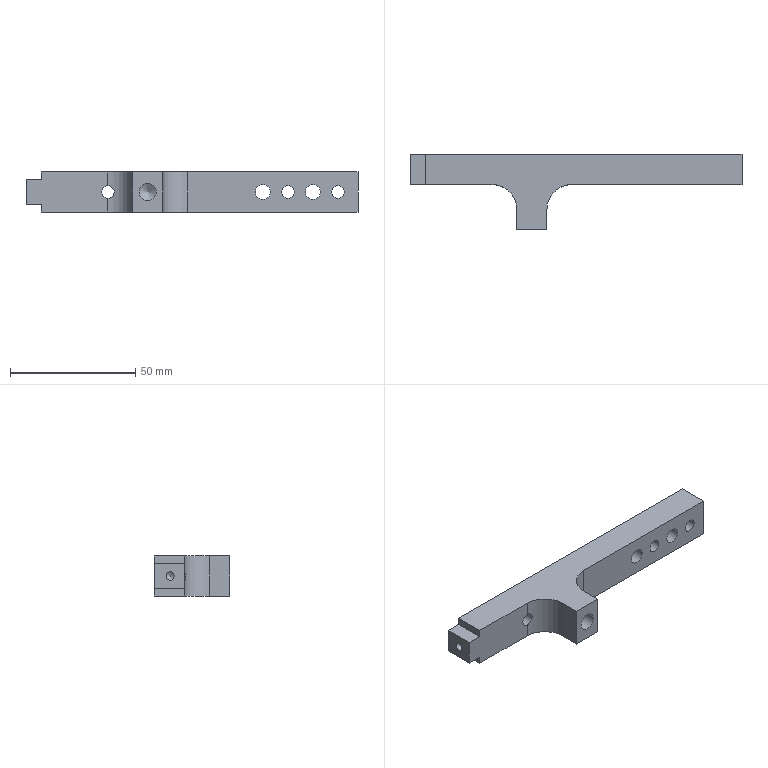Part | NX | features BREP 1 | 1 solid | 25 faces | box 132.75 x 30 x 16 mm | volume 26981 mm3 | plane 14 | cylinder 9 | cone 2 | commonest cylinder face diameters 5 x3 6 x2 20 x2 3.3 x1 6.8 x1
STEP:
#1=CARTESIAN_POINT('',(-36.75,30.,3.));
#2=VERTEX_POINT('',#1);
#3=CARTESIAN_POINT('',(-36.75,30.,0.));
#4=VERTEX_POINT('',#3);
#5=CARTESIAN_POINT('',(-36.75,30.,16.));
#6=DIRECTION('',(0.,0.,-1.));
#7=VECTOR('',#6,1000.);
#8=LINE('',#5,#7);
#9=EDGE_CURVE('',#2,#4,#8,.T.);
#10=ORIENTED_EDGE('',*,*,#9,.F.);
#11=CARTESIAN_POINT('',(-42.75,30.,3.));
#12=VERTEX_POINT('',#11);
#13=CARTESIAN_POINT('',(0.,30.,3.));
#14=DIRECTION('',(1.,0.,0.));
#15=VECTOR('',#14,1000.);
#16=LINE('',#13,#15);
#17=EDGE_CURVE('',#12,#2,#16,.T.);
#18=ORIENTED_EDGE('',*,*,#17,.F.);
#19=CARTESIAN_POINT('',(-42.75,30.,13.));
#20=VERTEX_POINT('',#19);
#21=CARTESIAN_POINT('',(-42.75,30.,16.));
#22=DIRECTION('',(0.,0.,-1.));
#23=VECTOR('',#22,1000.);
#24=LINE('',#21,#23);
#25=EDGE_CURVE('',#20,#12,#24,.T.);
#26=ORIENTED_EDGE('',*,*,#25,.F.);
#27=CARTESIAN_POINT('',(-36.75,30.,13.));
#28=VERTEX_POINT('',#27);
#29=CARTESIAN_POINT('',(0.,30.,13.));
#30=DIRECTION('',(-1.,0.,0.));
#31=VECTOR('',#30,1000.);
#32=LINE('',#29,#31);
#33=EDGE_CURVE('',#28,#20,#32,.T.);
#34=ORIENTED_EDGE('',*,*,#33,.F.);
#35=CARTESIAN_POINT('',(-36.75,30.,16.));
#36=VERTEX_POINT('',#35);
#37=CARTESIAN_POINT('',(-36.75,30.,16.));
#38=DIRECTION('',(0.,0.,-1.));
#39=VECTOR('',#38,1000.);
#40=LINE('',#37,#39);
#41=EDGE_CURVE('',#36,#28,#40,.T.);
#42=ORIENTED_EDGE('',*,*,#41,.F.);
#43=CARTESIAN_POINT('',(90.,30.,16.));
#44=VERTEX_POINT('',#43);
#45=CARTESIAN_POINT('',(0.,30.,16.));
#46=DIRECTION('',(-1.,0.,0.));
#47=VECTOR('',#46,1000.);
#48=LINE('',#45,#47);
#49=EDGE_CURVE('',#44,#36,#48,.T.);
#50=ORIENTED_EDGE('',*,*,#49,.F.);
#51=CARTESIAN_POINT('',(90.,30.,0.));
#52=VERTEX_POINT('',#51);
#53=CARTESIAN_POINT('',(90.,30.,16.));
#54=DIRECTION('',(0.,0.,1.));
#55=VECTOR('',#54,1000.);
#56=LINE('',#53,#55);
#57=EDGE_CURVE('',#52,#44,#56,.T.);
#58=ORIENTED_EDGE('',*,*,#57,.F.);
#59=CARTESIAN_POINT('',(0.,30.,0.));
#60=DIRECTION('',(1.,0.,0.));
#61=VECTOR('',#60,1000.);
#62=LINE('',#59,#61);
#63=EDGE_CURVE('',#4,#52,#62,.T.);
#64=ORIENTED_EDGE('',*,*,#63,.F.);
#65=EDGE_LOOP('',(#10,#18,#26,#34,#42,#50,#58,#64));
#66=FACE_BOUND('',#65,.T.);
#67=CARTESIAN_POINT('',(72.,30.,11.));
#68=VERTEX_POINT('',#67);
#69=CARTESIAN_POINT('',(72.,30.,8.));
#70=DIRECTION('',(0.,1.,0.));
#71=DIRECTION('',(0.,0.,1.));
#72=AXIS2_PLACEMENT_3D('',#69,#70,#71);
#73=CIRCLE('',#72,3.);
#74=EDGE_CURVE('',#68,#68,#73,.T.);
#75=ORIENTED_EDGE('',*,*,#74,.F.);
#76=EDGE_LOOP('',(#75));
#77=FACE_BOUND('',#76,.T.);
#78=CARTESIAN_POINT('',(52.,30.,11.));
#79=VERTEX_POINT('',#78);
#80=CARTESIAN_POINT('',(52.,30.,8.));
#81=DIRECTION('',(0.,1.,0.));
#82=DIRECTION('',(0.,0.,1.));
#83=AXIS2_PLACEMENT_3D('',#80,#81,#82);
#84=CIRCLE('',#83,3.);
#85=EDGE_CURVE('',#79,#79,#84,.T.);
#86=ORIENTED_EDGE('',*,*,#85,.F.);
#87=EDGE_LOOP('',(#86));
#88=FACE_BOUND('',#87,.T.);
#89=CARTESIAN_POINT('',(62.,30.,10.5));
#90=VERTEX_POINT('',#89);
#91=CARTESIAN_POINT('',(62.,30.,8.));
#92=DIRECTION('',(0.,1.,0.));
#93=DIRECTION('',(0.,0.,1.));
#94=AXIS2_PLACEMENT_3D('',#91,#92,#93);
#95=CIRCLE('',#94,2.5);
#96=EDGE_CURVE('',#90,#90,#95,.T.);
#97=ORIENTED_EDGE('',*,*,#96,.F.);
#98=EDGE_LOOP('',(#97));
#99=FACE_BOUND('',#98,.T.);
#100=CARTESIAN_POINT('',(82.,30.,10.5));
#101=VERTEX_POINT('',#100);
#102=CARTESIAN_POINT('',(82.,30.,8.));
#103=DIRECTION('',(0.,1.,0.));
#104=DIRECTION('',(0.,0.,1.));
#105=AXIS2_PLACEMENT_3D('',#102,#103,#104);
#106=CIRCLE('',#105,2.5);
#107=EDGE_CURVE('',#101,#101,#106,.T.);
#108=ORIENTED_EDGE('',*,*,#107,.F.);
#109=EDGE_LOOP('',(#108));
#110=FACE_BOUND('',#109,.T.);
#111=CARTESIAN_POINT('',(-10.,30.,10.5));
#112=VERTEX_POINT('',#111);
#113=CARTESIAN_POINT('',(-10.,30.,8.));
#114=DIRECTION('',(0.,1.,0.));
#115=DIRECTION('',(0.,0.,1.));
#116=AXIS2_PLACEMENT_3D('',#113,#114,#115);
#117=CIRCLE('',#116,2.5);
#118=EDGE_CURVE('',#112,#112,#117,.T.);
#119=ORIENTED_EDGE('',*,*,#118,.F.);
#120=EDGE_LOOP('',(#119));
#121=FACE_BOUND('',#120,.T.);
#122=CARTESIAN_POINT('',(0.,30.,16.));
#123=DIRECTION('',(0.,-1.,0.));
#124=DIRECTION('',(0.,0.,1.));
#125=AXIS2_PLACEMENT_3D('',#122,#123,#124);
#126=PLANE('',#125);
#127=ADVANCED_FACE('',(#66,#77,#88,#99,#110,#121),#126,.F.);
#128=CARTESIAN_POINT('',(0.,8.,0.));
#129=VERTEX_POINT('',#128);
#130=CARTESIAN_POINT('',(-10.,18.,0.));
#131=VERTEX_POINT('',#130);
#132=CARTESIAN_POINT('',(-10.,8.,0.));
#133=DIRECTION('',(0.,0.,1.));
#134=DIRECTION('',(-1.,0.,0.));
#135=AXIS2_PLACEMENT_3D('',#132,#133,#134);
#136=CIRCLE('',#135,10.);
#137=EDGE_CURVE('',#129,#131,#136,.T.);
#138=ORIENTED_EDGE('',*,*,#137,.T.);
#139=CARTESIAN_POINT('',(-36.75,18.,0.));
#140=VERTEX_POINT('',#139);
#141=CARTESIAN_POINT('',(0.,18.,0.));
#142=DIRECTION('',(-1.,0.,0.));
#143=VECTOR('',#142,1000.);
#144=LINE('',#141,#143);
#145=EDGE_CURVE('',#131,#140,#144,.T.);
#146=ORIENTED_EDGE('',*,*,#145,.T.);
#147=CARTESIAN_POINT('',(-36.75,0.,0.));
#148=DIRECTION('',(0.,1.,0.));
#149=VECTOR('',#148,1000.);
#150=LINE('',#147,#149);
#151=EDGE_CURVE('',#140,#4,#150,.T.);
#152=ORIENTED_EDGE('',*,*,#151,.T.);
#153=ORIENTED_EDGE('',*,*,#63,.T.);
#154=CARTESIAN_POINT('',(90.,18.,0.));
#155=VERTEX_POINT('',#154);
#156=CARTESIAN_POINT('',(90.,0.,0.));
#157=DIRECTION('',(0.,-1.,0.));
#158=VECTOR('',#157,1000.);
#159=LINE('',#156,#158);
#160=EDGE_CURVE('',#52,#155,#159,.T.);
#161=ORIENTED_EDGE('',*,*,#160,.T.);
#162=CARTESIAN_POINT('',(22.,18.,0.));
#163=VERTEX_POINT('',#162);
#164=CARTESIAN_POINT('',(0.,18.,0.));
#165=DIRECTION('',(-1.,0.,0.));
#166=VECTOR('',#165,1000.);
#167=LINE('',#164,#166);
#168=EDGE_CURVE('',#155,#163,#167,.T.);
#169=ORIENTED_EDGE('',*,*,#168,.T.);
#170=CARTESIAN_POINT('',(12.,8.,0.));
#171=VERTEX_POINT('',#170);
#172=CARTESIAN_POINT('',(22.,8.,0.));
#173=DIRECTION('',(0.,0.,1.));
#174=DIRECTION('',(1.,0.,0.));
#175=AXIS2_PLACEMENT_3D('',#172,#173,#174);
#176=CIRCLE('',#175,10.);
#177=EDGE_CURVE('',#163,#171,#176,.T.);
#178=ORIENTED_EDGE('',*,*,#177,.T.);
#179=CARTESIAN_POINT('',(12.,0.,0.));
#180=VERTEX_POINT('',#179);
#181=CARTESIAN_POINT('',(12.,0.,0.));
#182=DIRECTION('',(0.,-1.,0.));
#183=VECTOR('',#182,1000.);
#184=LINE('',#181,#183);
#185=EDGE_CURVE('',#171,#180,#184,.T.);
#186=ORIENTED_EDGE('',*,*,#185,.T.);
#187=CARTESIAN_POINT('',(0.,0.,0.));
#188=VERTEX_POINT('',#187);
#189=CARTESIAN_POINT('',(0.,0.,0.));
#190=DIRECTION('',(-1.,0.,0.));
#191=VECTOR('',#190,1000.);
#192=LINE('',#189,#191);
#193=EDGE_CURVE('',#180,#188,#192,.T.);
#194=ORIENTED_EDGE('',*,*,#193,.T.);
#195=CARTESIAN_POINT('',(0.,0.,0.));
#196=DIRECTION('',(0.,1.,0.));
#197=VECTOR('',#196,1000.);
#198=LINE('',#195,#197);
#199=EDGE_CURVE('',#188,#129,#198,.T.);
#200=ORIENTED_EDGE('',*,*,#199,.T.);
#201=EDGE_LOOP('',(#138,#146,#152,#153,#161,#169,#178,#186,#194,#200));
#202=FACE_BOUND('',#201,.T.);
#203=CARTESIAN_POINT('',(0.,0.,0.));
#204=DIRECTION('',(0.,0.,-1.));
#205=DIRECTION('',(1.,0.,0.));
#206=AXIS2_PLACEMENT_3D('',#203,#204,#205);
#207=PLANE('',#206);
#208=ADVANCED_FACE('',(#202),#207,.T.);
#209=CARTESIAN_POINT('',(-36.75,18.,3.));
#210=VERTEX_POINT('',#209);
#211=CARTESIAN_POINT('',(-36.75,0.,3.));
#212=DIRECTION('',(0.,-1.,0.));
#213=VECTOR('',#212,1000.);
#214=LINE('',#211,#213);
#215=EDGE_CURVE('',#2,#210,#214,.T.);
#216=ORIENTED_EDGE('',*,*,#215,.F.);
#217=ORIENTED_EDGE('',*,*,#9,.T.);
#218=ORIENTED_EDGE('',*,*,#151,.F.);
#219=CARTESIAN_POINT('',(-36.75,18.,0.));
#220=DIRECTION('',(0.,0.,-1.));
#221=VECTOR('',#220,1000.);
#222=LINE('',#219,#221);
#223=EDGE_CURVE('',#210,#140,#222,.T.);
#224=ORIENTED_EDGE('',*,*,#223,.F.);
#225=EDGE_LOOP('',(#216,#217,#218,#224));
#226=FACE_BOUND('',#225,.T.);
#227=CARTESIAN_POINT('',(-36.75,0.,0.));
#228=DIRECTION('',(1.,0.,0.));
#229=DIRECTION('',(0.,0.,1.));
#230=AXIS2_PLACEMENT_3D('',#227,#228,#229);
#231=PLANE('',#230);
#232=ADVANCED_FACE('',(#226),#231,.F.);
#233=CARTESIAN_POINT('',(-42.75,18.,3.));
#234=VERTEX_POINT('',#233);
#235=CARTESIAN_POINT('',(-42.75,0.,3.));
#236=DIRECTION('',(0.,-1.,0.));
#237=VECTOR('',#236,1000.);
#238=LINE('',#235,#237);
#239=EDGE_CURVE('',#12,#234,#238,.T.);
#240=ORIENTED_EDGE('',*,*,#239,.F.);
#241=ORIENTED_EDGE('',*,*,#17,.T.);
#242=ORIENTED_EDGE('',*,*,#215,.T.);
#243=CARTESIAN_POINT('',(-36.75,18.,3.));
#244=DIRECTION('',(1.,0.,0.));
#245=VECTOR('',#244,1000.);
#246=LINE('',#243,#245);
#247=EDGE_CURVE('',#234,#210,#246,.T.);
#248=ORIENTED_EDGE('',*,*,#247,.F.);
#249=EDGE_LOOP('',(#240,#241,#242,#248));
#250=FACE_BOUND('',#249,.T.);
#251=CARTESIAN_POINT('',(-36.75,0.,3.));
#252=DIRECTION('',(0.,0.,1.));
#253=DIRECTION('',(-1.,0.,0.));
#254=AXIS2_PLACEMENT_3D('',#251,#252,#253);
#255=PLANE('',#254);
#256=ADVANCED_FACE('',(#250),#255,.F.);
#257=CARTESIAN_POINT('',(-42.75,18.,13.));
#258=VERTEX_POINT('',#257);
#259=CARTESIAN_POINT('',(-42.75,30.,13.));
#260=DIRECTION('',(0.,1.,0.));
#261=VECTOR('',#260,1000.);
#262=LINE('',#259,#261);
#263=EDGE_CURVE('',#258,#20,#262,.T.);
#264=ORIENTED_EDGE('',*,*,#263,.T.);
#265=ORIENTED_EDGE('',*,*,#25,.T.);
#266=ORIENTED_EDGE('',*,*,#239,.T.);
#267=CARTESIAN_POINT('',(-42.75,18.,16.));
#268=DIRECTION('',(0.,0.,1.));
#269=VECTOR('',#268,1000.);
#270=LINE('',#267,#269);
#271=EDGE_CURVE('',#234,#258,#270,.T.);
#272=ORIENTED_EDGE('',*,*,#271,.T.);
#273=EDGE_LOOP('',(#264,#265,#266,#272));
#274=FACE_BOUND('',#273,.T.);
#275=CARTESIAN_POINT('',(-42.75,23.75,9.65));
#276=VERTEX_POINT('',#275);
#277=CARTESIAN_POINT('',(-42.75,23.75,8.));
#278=DIRECTION('',(1.,0.,0.));
#279=DIRECTION('',(0.,0.,1.));
#280=AXIS2_PLACEMENT_3D('',#277,#278,#279);
#281=CIRCLE('',#280,1.65);
#282=EDGE_CURVE('',#276,#276,#281,.T.);
#283=ORIENTED_EDGE('',*,*,#282,.T.);
#284=EDGE_LOOP('',(#283));
#285=FACE_BOUND('',#284,.T.);
#286=CARTESIAN_POINT('',(-42.75,30.,16.));
#287=DIRECTION('',(-1.,0.,0.));
#288=DIRECTION('',(0.,1.,0.));
#289=AXIS2_PLACEMENT_3D('',#286,#287,#288);
#290=PLANE('',#289);
#291=ADVANCED_FACE('',(#274,#285),#290,.T.);
#292=CARTESIAN_POINT('',(-36.75,18.,13.));
#293=VERTEX_POINT('',#292);
#294=CARTESIAN_POINT('',(-36.75,0.,13.));
#295=DIRECTION('',(0.,-1.,0.));
#296=VECTOR('',#295,1000.);
#297=LINE('',#294,#296);
#298=EDGE_CURVE('',#28,#293,#297,.T.);
#299=ORIENTED_EDGE('',*,*,#298,.F.);
#300=ORIENTED_EDGE('',*,*,#33,.T.);
#301=ORIENTED_EDGE('',*,*,#263,.F.);
#302=CARTESIAN_POINT('',(-36.75,18.,13.));
#303=DIRECTION('',(-1.,0.,0.));
#304=VECTOR('',#303,1000.);
#305=LINE('',#302,#304);
#306=EDGE_CURVE('',#293,#258,#305,.T.);
#307=ORIENTED_EDGE('',*,*,#306,.F.);
#308=EDGE_LOOP('',(#299,#300,#301,#307));
#309=FACE_BOUND('',#308,.T.);
#310=CARTESIAN_POINT('',(-36.75,0.,13.));
#311=DIRECTION('',(0.,0.,-1.));
#312=DIRECTION('',(1.,0.,0.));
#313=AXIS2_PLACEMENT_3D('',#310,#311,#312);
#314=PLANE('',#313);
#315=ADVANCED_FACE('',(#309),#314,.F.);
#316=CARTESIAN_POINT('',(-36.75,18.,16.));
#317=VERTEX_POINT('',#316);
#318=CARTESIAN_POINT('',(-36.75,0.,16.));
#319=DIRECTION('',(0.,-1.,0.));
#320=VECTOR('',#319,1000.);
#321=LINE('',#318,#320);
#322=EDGE_CURVE('',#36,#317,#321,.T.);
#323=ORIENTED_EDGE('',*,*,#322,.F.);
#324=ORIENTED_EDGE('',*,*,#41,.T.);
#325=ORIENTED_EDGE('',*,*,#298,.T.);
#326=CARTESIAN_POINT('',(-36.75,18.,16.));
#327=DIRECTION('',(0.,0.,-1.));
#328=VECTOR('',#327,1000.);
#329=LINE('',#326,#328);
#330=EDGE_CURVE('',#317,#293,#329,.T.);
#331=ORIENTED_EDGE('',*,*,#330,.F.);
#332=EDGE_LOOP('',(#323,#324,#325,#331));
#333=FACE_BOUND('',#332,.T.);
#334=CARTESIAN_POINT('',(-36.75,0.,16.));
#335=DIRECTION('',(1.,0.,0.));
#336=DIRECTION('',(0.,0.,1.));
#337=AXIS2_PLACEMENT_3D('',#334,#335,#336);
#338=PLANE('',#337);
#339=ADVANCED_FACE('',(#333),#338,.F.);
#340=ORIENTED_EDGE('',*,*,#322,.T.);
#341=CARTESIAN_POINT('',(-10.,18.,16.));
#342=VERTEX_POINT('',#341);
#343=CARTESIAN_POINT('',(0.,18.,16.));
#344=DIRECTION('',(-1.,0.,0.));
#345=VECTOR('',#344,1000.);
#346=LINE('',#343,#345);
#347=EDGE_CURVE('',#342,#317,#346,.T.);
#348=ORIENTED_EDGE('',*,*,#347,.F.);
#349=CARTESIAN_POINT('',(0.,8.,16.));
#350=VERTEX_POINT('',#349);
#351=CARTESIAN_POINT('',(-10.,8.,16.));
#352=DIRECTION('',(0.,0.,1.));
#353=DIRECTION('',(-1.,0.,0.));
#354=AXIS2_PLACEMENT_3D('',#351,#352,#353);
#355=CIRCLE('',#354,10.);
#356=EDGE_CURVE('',#350,#342,#355,.T.);
#357=ORIENTED_EDGE('',*,*,#356,.F.);
#358=CARTESIAN_POINT('',(0.,0.,16.));
#359=VERTEX_POINT('',#358);
#360=CARTESIAN_POINT('',(0.,0.,16.));
#361=DIRECTION('',(0.,1.,0.));
#362=VECTOR('',#361,1000.);
#363=LINE('',#360,#362);
#364=EDGE_CURVE('',#359,#350,#363,.T.);
#365=ORIENTED_EDGE('',*,*,#364,.F.);
#366=CARTESIAN_POINT('',(12.,0.,16.));
#367=VERTEX_POINT('',#366);
#368=CARTESIAN_POINT('',(0.,0.,16.));
#369=DIRECTION('',(-1.,0.,0.));
#370=VECTOR('',#369,1000.);
#371=LINE('',#368,#370);
#372=EDGE_CURVE('',#367,#359,#371,.T.);
#373=ORIENTED_EDGE('',*,*,#372,.F.);
#374=CARTESIAN_POINT('',(12.,8.,16.));
#375=VERTEX_POINT('',#374);
#376=CARTESIAN_POINT('',(12.,0.,16.));
#377=DIRECTION('',(0.,-1.,0.));
#378=VECTOR('',#377,1000.);
#379=LINE('',#376,#378);
#380=EDGE_CURVE('',#375,#367,#379,.T.);
#381=ORIENTED_EDGE('',*,*,#380,.F.);
#382=CARTESIAN_POINT('',(22.,18.,16.));
#383=VERTEX_POINT('',#382);
#384=CARTESIAN_POINT('',(22.,8.,16.));
#385=DIRECTION('',(0.,0.,1.));
#386=DIRECTION('',(1.,0.,0.));
#387=AXIS2_PLACEMENT_3D('',#384,#385,#386);
#388=CIRCLE('',#387,10.);
#389=EDGE_CURVE('',#383,#375,#388,.T.);
#390=ORIENTED_EDGE('',*,*,#389,.F.);
#391=CARTESIAN_POINT('',(90.,18.,16.));
#392=VERTEX_POINT('',#391);
#393=CARTESIAN_POINT('',(0.,18.,16.));
#394=DIRECTION('',(-1.,0.,0.));
#395=VECTOR('',#394,1000.);
#396=LINE('',#393,#395);
#397=EDGE_CURVE('',#392,#383,#396,.T.);
#398=ORIENTED_EDGE('',*,*,#397,.F.);
#399=CARTESIAN_POINT('',(90.,0.,16.));
#400=DIRECTION('',(0.,-1.,0.));
#401=VECTOR('',#400,1000.);
#402=LINE('',#399,#401);
#403=EDGE_CURVE('',#44,#392,#402,.T.);
#404=ORIENTED_EDGE('',*,*,#403,.F.);
#405=ORIENTED_EDGE('',*,*,#49,.T.);
#406=EDGE_LOOP('',(#340,#348,#357,#365,#373,#381,#390,#398,#404,#405));
#407=FACE_BOUND('',#406,.T.);
#408=CARTESIAN_POINT('',(0.,0.,16.));
#409=DIRECTION('',(0.,0.,-1.));
#410=DIRECTION('',(1.,0.,0.));
#411=AXIS2_PLACEMENT_3D('',#408,#409,#410);
#412=PLANE('',#411);
#413=ADVANCED_FACE('',(#407),#412,.F.);
#414=ORIENTED_EDGE('',*,*,#57,.T.);
#415=ORIENTED_EDGE('',*,*,#403,.T.);
#416=CARTESIAN_POINT('',(90.,18.,16.));
#417=DIRECTION('',(0.,0.,1.));
#418=VECTOR('',#417,1000.);
#419=LINE('',#416,#418);
#420=EDGE_CURVE('',#155,#392,#419,.T.);
#421=ORIENTED_EDGE('',*,*,#420,.F.);
#422=ORIENTED_EDGE('',*,*,#160,.F.);
#423=EDGE_LOOP('',(#414,#415,#421,#422));
#424=FACE_BOUND('',#423,.T.);
#425=CARTESIAN_POINT('',(90.,30.,16.));
#426=DIRECTION('',(-1.,0.,0.));
#427=DIRECTION('',(0.,0.,-1.));
#428=AXIS2_PLACEMENT_3D('',#425,#426,#427);
#429=PLANE('',#428);
#430=ADVANCED_FACE('',(#424),#429,.F.);
#431=CARTESIAN_POINT('',(72.,18.,11.));
#432=VERTEX_POINT('',#431);
#433=CARTESIAN_POINT('',(72.,18.,8.));
#434=DIRECTION('',(0.,1.,0.));
#435=DIRECTION('',(0.,0.,1.));
#436=AXIS2_PLACEMENT_3D('',#433,#434,#435);
#437=CIRCLE('',#436,3.);
#438=EDGE_CURVE('',#432,#432,#437,.T.);
#439=ORIENTED_EDGE('',*,*,#438,.F.);
#440=EDGE_LOOP('',(#439));
#441=FACE_BOUND('',#440,.T.);
#442=ORIENTED_EDGE('',*,*,#74,.T.);
#443=EDGE_LOOP('',(#442));
#444=FACE_BOUND('',#443,.T.);
#445=CARTESIAN_POINT('',(72.,30.,8.));
#446=DIRECTION('',(0.,1.,0.));
#447=DIRECTION('',(0.,0.,-1.));
#448=AXIS2_PLACEMENT_3D('',#445,#446,#447);
#449=CYLINDRICAL_SURFACE('',#448,3.);
#450=ADVANCED_FACE('',(#441,#444),#449,.F.);
#451=CARTESIAN_POINT('',(52.,18.,11.));
#452=VERTEX_POINT('',#451);
#453=CARTESIAN_POINT('',(52.,18.,8.));
#454=DIRECTION('',(0.,1.,0.));
#455=DIRECTION('',(0.,0.,1.));
#456=AXIS2_PLACEMENT_3D('',#453,#454,#455);
#457=CIRCLE('',#456,3.);
#458=EDGE_CURVE('',#452,#452,#457,.T.);
#459=ORIENTED_EDGE('',*,*,#458,.F.);
#460=EDGE_LOOP('',(#459));
#461=FACE_BOUND('',#460,.T.);
#462=ORIENTED_EDGE('',*,*,#85,.T.);
#463=EDGE_LOOP('',(#462));
#464=FACE_BOUND('',#463,.T.);
#465=CARTESIAN_POINT('',(52.,30.,8.));
#466=DIRECTION('',(0.,1.,0.));
#467=DIRECTION('',(0.,0.,-1.));
#468=AXIS2_PLACEMENT_3D('',#465,#466,#467);
#469=CYLINDRICAL_SURFACE('',#468,3.);
#470=ADVANCED_FACE('',(#461,#464),#469,.F.);
#471=CARTESIAN_POINT('',(62.,18.,10.5));
#472=VERTEX_POINT('',#471);
#473=CARTESIAN_POINT('',(62.,18.,8.));
#474=DIRECTION('',(0.,1.,0.));
#475=DIRECTION('',(0.,0.,1.));
#476=AXIS2_PLACEMENT_3D('',#473,#474,#475);
#477=CIRCLE('',#476,2.5);
#478=EDGE_CURVE('',#472,#472,#477,.T.);
#479=ORIENTED_EDGE('',*,*,#478,.F.);
#480=EDGE_LOOP('',(#479));
#481=FACE_BOUND('',#480,.T.);
#482=ORIENTED_EDGE('',*,*,#96,.T.);
#483=EDGE_LOOP('',(#482));
#484=FACE_BOUND('',#483,.T.);
#485=CARTESIAN_POINT('',(62.,30.,8.));
#486=DIRECTION('',(0.,1.,0.));
#487=DIRECTION('',(0.,0.,-1.));
#488=AXIS2_PLACEMENT_3D('',#485,#486,#487);
#489=CYLINDRICAL_SURFACE('',#488,2.5);
#490=ADVANCED_FACE('',(#481,#484),#489,.F.);
#491=CARTESIAN_POINT('',(82.,18.,10.5));
#492=VERTEX_POINT('',#491);
#493=CARTESIAN_POINT('',(82.,18.,8.));
#494=DIRECTION('',(0.,1.,0.));
#495=DIRECTION('',(0.,0.,1.));
#496=AXIS2_PLACEMENT_3D('',#493,#494,#495);
#497=CIRCLE('',#496,2.5);
#498=EDGE_CURVE('',#492,#492,#497,.T.);
#499=ORIENTED_EDGE('',*,*,#498,.F.);
#500=EDGE_LOOP('',(#499));
#501=FACE_BOUND('',#500,.T.);
#502=ORIENTED_EDGE('',*,*,#107,.T.);
#503=EDGE_LOOP('',(#502));
#504=FACE_BOUND('',#503,.T.);
#505=CARTESIAN_POINT('',(82.,30.,8.));
#506=DIRECTION('',(0.,1.,0.));
#507=DIRECTION('',(0.,0.,-1.));
#508=AXIS2_PLACEMENT_3D('',#505,#506,#507);
#509=CYLINDRICAL_SURFACE('',#508,2.5);
#510=ADVANCED_FACE('',(#501,#504),#509,.F.);
#511=CARTESIAN_POINT('',(-10.,18.,10.5));
#512=VERTEX_POINT('',#511);
#513=CARTESIAN_POINT('',(-10.,18.,5.5));
#514=VERTEX_POINT('',#513);
#515=CARTESIAN_POINT('',(-10.,18.,10.5));
#516=CARTESIAN_POINT('',(-9.337,18.,10.5));
#517=CARTESIAN_POINT('',(-8.046,17.844,9.958));
#518=CARTESIAN_POINT('',(-7.227,17.602,8.004));
#519=CARTESIAN_POINT('',(-8.044,17.843,6.041));
#520=CARTESIAN_POINT('',(-9.337,18.,5.5));
#521=CARTESIAN_POINT('',(-10.,18.,5.5));
#522=B_SPLINE_CURVE_WITH_KNOTS('',3,(#515,#516,#517,#518,#519,#520,#521),.UNSPECIFIED.,.F.,.F.,(4,1,1,1,4),(0.,0.001961,0.003922,0.005884,0.007845),.UNSPECIFIED.);
#523=EDGE_CURVE('',#512,#514,#522,.T.);
#524=ORIENTED_EDGE('',*,*,#523,.F.);
#525=CARTESIAN_POINT('',(-10.,18.,8.));
#526=DIRECTION('',(0.,1.,0.));
#527=DIRECTION('',(0.,0.,1.));
#528=AXIS2_PLACEMENT_3D('',#525,#526,#527);
#529=CIRCLE('',#528,2.5);
#530=EDGE_CURVE('',#514,#512,#529,.T.);
#531=ORIENTED_EDGE('',*,*,#530,.F.);
#532=EDGE_LOOP('',(#524,#531));
#533=FACE_BOUND('',#532,.T.);
#534=ORIENTED_EDGE('',*,*,#118,.T.);
#535=EDGE_LOOP('',(#534));
#536=FACE_BOUND('',#535,.T.);
#537=CARTESIAN_POINT('',(-10.,30.,8.));
#538=DIRECTION('',(0.,1.,0.));
#539=DIRECTION('',(0.,0.,-1.));
#540=AXIS2_PLACEMENT_3D('',#537,#538,#539);
#541=CYLINDRICAL_SURFACE('',#540,2.5);
#542=ADVANCED_FACE('',(#533,#536),#541,.F.);
#543=ORIENTED_EDGE('',*,*,#145,.F.);
#544=CARTESIAN_POINT('',(-10.,18.,16.));
#545=DIRECTION('',(0.,0.,1.));
#546=VECTOR('',#545,1000.);
#547=LINE('',#544,#546);
#548=EDGE_CURVE('',#131,#514,#547,.T.);
#549=ORIENTED_EDGE('',*,*,#548,.T.);
#550=ORIENTED_EDGE('',*,*,#530,.T.);
#551=CARTESIAN_POINT('',(-10.,18.,16.));
#552=DIRECTION('',(0.,0.,1.));
#553=VECTOR('',#552,1000.);
#554=LINE('',#551,#553);
#555=EDGE_CURVE('',#512,#342,#554,.T.);
#556=ORIENTED_EDGE('',*,*,#555,.T.);
#557=ORIENTED_EDGE('',*,*,#347,.T.);
#558=ORIENTED_EDGE('',*,*,#330,.T.);
#559=ORIENTED_EDGE('',*,*,#306,.T.);
#560=ORIENTED_EDGE('',*,*,#271,.F.);
#561=ORIENTED_EDGE('',*,*,#247,.T.);
#562=ORIENTED_EDGE('',*,*,#223,.T.);
#563=EDGE_LOOP('',(#543,#549,#550,#556,#557,#558,#559,#560,#561,#562));
#564=FACE_BOUND('',#563,.T.);
#565=CARTESIAN_POINT('',(-42.75,18.,16.));
#566=DIRECTION('',(0.,-1.,0.));
#567=DIRECTION('',(-1.,0.,0.));
#568=AXIS2_PLACEMENT_3D('',#565,#566,#567);
#569=PLANE('',#568);
#570=ADVANCED_FACE('',(#564),#569,.T.);
#571=ORIENTED_EDGE('',*,*,#523,.T.);
#572=ORIENTED_EDGE('',*,*,#548,.F.);
#573=ORIENTED_EDGE('',*,*,#137,.F.);
#574=CARTESIAN_POINT('',(0.,8.,16.));
#575=DIRECTION('',(0.,0.,-1.));
#576=VECTOR('',#575,1000.);
#577=LINE('',#574,#576);
#578=EDGE_CURVE('',#350,#129,#577,.T.);
#579=ORIENTED_EDGE('',*,*,#578,.F.);
#580=ORIENTED_EDGE('',*,*,#356,.T.);
#581=ORIENTED_EDGE('',*,*,#555,.F.);
#582=EDGE_LOOP('',(#571,#572,#573,#579,#580,#581));
#583=FACE_BOUND('',#582,.T.);
#584=CARTESIAN_POINT('',(-10.,8.,16.));
#585=DIRECTION('',(0.,0.,-1.));
#586=DIRECTION('',(1.,0.,0.));
#587=AXIS2_PLACEMENT_3D('',#584,#585,#586);
#588=CYLINDRICAL_SURFACE('',#587,10.);
#589=ADVANCED_FACE('',(#583),#588,.F.);
#590=ORIENTED_EDGE('',*,*,#578,.T.);
#591=ORIENTED_EDGE('',*,*,#199,.F.);
#592=CARTESIAN_POINT('',(0.,0.,16.));
#593=DIRECTION('',(0.,0.,-1.));
#594=VECTOR('',#593,1000.);
#595=LINE('',#592,#594);
#596=EDGE_CURVE('',#359,#188,#595,.T.);
#597=ORIENTED_EDGE('',*,*,#596,.F.);
#598=ORIENTED_EDGE('',*,*,#364,.T.);
#599=EDGE_LOOP('',(#590,#591,#597,#598));
#600=FACE_BOUND('',#599,.T.);
#601=CARTESIAN_POINT('',(0.,0.,16.));
#602=DIRECTION('',(1.,0.,0.));
#603=DIRECTION('',(0.,0.,1.));
#604=AXIS2_PLACEMENT_3D('',#601,#602,#603);
#605=PLANE('',#604);
#606=ADVANCED_FACE('',(#600),#605,.F.);
#607=CARTESIAN_POINT('',(12.,0.,16.));
#608=DIRECTION('',(0.,0.,-1.));
#609=VECTOR('',#608,1000.);
#610=LINE('',#607,#609);
#611=EDGE_CURVE('',#367,#180,#610,.T.);
#612=ORIENTED_EDGE('',*,*,#611,.F.);
#613=ORIENTED_EDGE('',*,*,#372,.T.);
#614=ORIENTED_EDGE('',*,*,#596,.T.);
#615=ORIENTED_EDGE('',*,*,#193,.F.);
#616=EDGE_LOOP('',(#612,#613,#614,#615));
#617=FACE_BOUND('',#616,.T.);
#618=CARTESIAN_POINT('',(6.,0.,4.6));
#619=VERTEX_POINT('',#618);
#620=CARTESIAN_POINT('',(6.,0.,8.));
#621=DIRECTION('',(0.,-1.,0.));
#622=DIRECTION('',(0.,0.,-1.));
#623=AXIS2_PLACEMENT_3D('',#620,#621,#622);
#624=CIRCLE('',#623,3.4);
#625=EDGE_CURVE('',#619,#619,#624,.T.);
#626=ORIENTED_EDGE('',*,*,#625,.F.);
#627=EDGE_LOOP('',(#626));
#628=FACE_BOUND('',#627,.T.);
#629=CARTESIAN_POINT('',(12.,0.,16.));
#630=DIRECTION('',(0.,1.,0.));
#631=DIRECTION('',(0.,0.,-1.));
#632=AXIS2_PLACEMENT_3D('',#629,#630,#631);
#633=PLANE('',#632);
#634=ADVANCED_FACE('',(#617,#628),#633,.F.);
#635=CARTESIAN_POINT('',(12.,8.,16.));
#636=DIRECTION('',(0.,0.,-1.));
#637=VECTOR('',#636,1000.);
#638=LINE('',#635,#637);
#639=EDGE_CURVE('',#375,#171,#638,.T.);
#640=ORIENTED_EDGE('',*,*,#639,.F.);
#641=ORIENTED_EDGE('',*,*,#380,.T.);
#642=ORIENTED_EDGE('',*,*,#611,.T.);
#643=ORIENTED_EDGE('',*,*,#185,.F.);
#644=EDGE_LOOP('',(#640,#641,#642,#643));
#645=FACE_BOUND('',#644,.T.);
#646=CARTESIAN_POINT('',(12.,18.,16.));
#647=DIRECTION('',(-1.,0.,0.));
#648=DIRECTION('',(0.,1.,0.));
#649=AXIS2_PLACEMENT_3D('',#646,#647,#648);
#650=PLANE('',#649);
#651=ADVANCED_FACE('',(#645),#650,.F.);
#652=ORIENTED_EDGE('',*,*,#639,.T.);
#653=ORIENTED_EDGE('',*,*,#177,.F.);
#654=CARTESIAN_POINT('',(22.,18.,16.));
#655=DIRECTION('',(0.,0.,-1.));
#656=VECTOR('',#655,1000.);
#657=LINE('',#654,#656);
#658=EDGE_CURVE('',#383,#163,#657,.T.);
#659=ORIENTED_EDGE('',*,*,#658,.F.);
#660=ORIENTED_EDGE('',*,*,#389,.T.);
#661=EDGE_LOOP('',(#652,#653,#659,#660));
#662=FACE_BOUND('',#661,.T.);
#663=CARTESIAN_POINT('',(22.,8.,16.));
#664=DIRECTION('',(0.,0.,1.));
#665=DIRECTION('',(-1.,0.,0.));
#666=AXIS2_PLACEMENT_3D('',#663,#664,#665);
#667=CYLINDRICAL_SURFACE('',#666,10.);
#668=ADVANCED_FACE('',(#662),#667,.F.);
#669=ORIENTED_EDGE('',*,*,#658,.T.);
#670=ORIENTED_EDGE('',*,*,#168,.F.);
#671=ORIENTED_EDGE('',*,*,#420,.T.);
#672=ORIENTED_EDGE('',*,*,#397,.T.);
#673=EDGE_LOOP('',(#669,#670,#671,#672));
#674=FACE_BOUND('',#673,.T.);
#675=ORIENTED_EDGE('',*,*,#438,.T.);
#676=EDGE_LOOP('',(#675));
#677=FACE_BOUND('',#676,.T.);
#678=ORIENTED_EDGE('',*,*,#458,.T.);
#679=EDGE_LOOP('',(#678));
#680=FACE_BOUND('',#679,.T.);
#681=ORIENTED_EDGE('',*,*,#478,.T.);
#682=EDGE_LOOP('',(#681));
#683=FACE_BOUND('',#682,.T.);
#684=ORIENTED_EDGE('',*,*,#498,.T.);
#685=EDGE_LOOP('',(#684));
#686=FACE_BOUND('',#685,.T.);
#687=CARTESIAN_POINT('',(90.,18.,16.));
#688=DIRECTION('',(0.,1.,0.));
#689=DIRECTION('',(1.,0.,0.));
#690=AXIS2_PLACEMENT_3D('',#687,#688,#689);
#691=PLANE('',#690);
#692=ADVANCED_FACE('',(#674,#677,#680,#683,#686),#691,.F.);
#693=ORIENTED_EDGE('',*,*,#282,.F.);
#694=EDGE_LOOP('',(#693));
#695=FACE_BOUND('',#694,.T.);
#696=CARTESIAN_POINT('',(-32.65,23.75,9.65));
#697=VERTEX_POINT('',#696);
#698=CARTESIAN_POINT('',(-32.65,23.75,8.));
#699=DIRECTION('',(-1.,0.,0.));
#700=DIRECTION('',(0.,0.,1.));
#701=AXIS2_PLACEMENT_3D('',#698,#699,#700);
#702=CIRCLE('',#701,1.65);
#703=EDGE_CURVE('',#697,#697,#702,.T.);
#704=ORIENTED_EDGE('',*,*,#703,.F.);
#705=EDGE_LOOP('',(#704));
#706=FACE_BOUND('',#705,.T.);
#707=CARTESIAN_POINT('',(-42.75,23.75,8.));
#708=DIRECTION('',(-1.,0.,0.));
#709=DIRECTION('',(0.,0.,-1.));
#710=AXIS2_PLACEMENT_3D('',#707,#708,#709);
#711=CYLINDRICAL_SURFACE('',#710,1.65);
#712=ADVANCED_FACE('',(#695,#706),#711,.F.);
#713=CARTESIAN_POINT('',(6.,19.75,4.6));
#714=VERTEX_POINT('',#713);
#715=CARTESIAN_POINT('',(6.,19.75,8.));
#716=DIRECTION('',(0.,-1.,0.));
#717=DIRECTION('',(0.,0.,-1.));
#718=AXIS2_PLACEMENT_3D('',#715,#716,#717);
#719=CIRCLE('',#718,3.4);
#720=EDGE_CURVE('',#714,#714,#719,.T.);
#721=ORIENTED_EDGE('',*,*,#720,.F.);
#722=EDGE_LOOP('',(#721));
#723=FACE_BOUND('',#722,.T.);
#724=ORIENTED_EDGE('',*,*,#625,.T.);
#725=EDGE_LOOP('',(#724));
#726=FACE_BOUND('',#725,.T.);
#727=CARTESIAN_POINT('',(6.,0.,8.));
#728=DIRECTION('',(0.,-1.,0.));
#729=DIRECTION('',(0.,0.,1.));
#730=AXIS2_PLACEMENT_3D('',#727,#728,#729);
#731=CYLINDRICAL_SURFACE('',#730,3.4);
#732=ADVANCED_FACE('',(#723,#726),#731,.F.);
#733=CARTESIAN_POINT('',(-31.659,23.75,8.));
#734=VERTEX_POINT('',#733);
#735=VERTEX_LOOP('',#734);
#736=FACE_BOUND('',#735,.T.);
#737=ORIENTED_EDGE('',*,*,#703,.T.);
#738=EDGE_LOOP('',(#737));
#739=FACE_BOUND('',#738,.T.);
#740=CARTESIAN_POINT('',(-32.65,23.75,8.));
#741=DIRECTION('',(-1.,0.,0.));
#742=DIRECTION('',(0.,0.,-1.));
#743=AXIS2_PLACEMENT_3D('',#740,#741,#742);
#744=CONICAL_SURFACE('',#743,1.65,1.03);
#745=ADVANCED_FACE('',(#736,#739),#744,.F.);
#746=CARTESIAN_POINT('',(6.,21.793,8.));
#747=VERTEX_POINT('',#746);
#748=VERTEX_LOOP('',#747);
#749=FACE_BOUND('',#748,.T.);
#750=ORIENTED_EDGE('',*,*,#720,.T.);
#751=EDGE_LOOP('',(#750));
#752=FACE_BOUND('',#751,.T.);
#753=CARTESIAN_POINT('',(6.,19.75,8.));
#754=DIRECTION('',(0.,-1.,0.));
#755=DIRECTION('',(0.,0.,1.));
#756=AXIS2_PLACEMENT_3D('',#753,#754,#755);
#757=CONICAL_SURFACE('',#756,3.4,1.03);
#758=ADVANCED_FACE('',(#749,#752),#757,.F.);
#759=CLOSED_SHELL('',(#127,#208,#232,#256,#291,#315,#339,#413,#430,#450,#470,#490,#510,#542,#570,#589,#606,#634,#651,#668,#692,#712,#732,#745,#758));
#760=MANIFOLD_SOLID_BREP('',#759);
#761=(LENGTH_UNIT()NAMED_UNIT(*)SI_UNIT(.MILLI.,.METRE.));
#762=UNCERTAINTY_MEASURE_WITH_UNIT(LENGTH_MEASURE(0.0508),#761,'','');
#763=(NAMED_UNIT(*)PLANE_ANGLE_UNIT()SI_UNIT($,.RADIAN.));
#764=(NAMED_UNIT(*)SI_UNIT($,.STERADIAN.)SOLID_ANGLE_UNIT());
#765=(GEOMETRIC_REPRESENTATION_CONTEXT(3)GLOBAL_UNCERTAINTY_ASSIGNED_CONTEXT((#762))GLOBAL_UNIT_ASSIGNED_CONTEXT((#761,#763,#764))REPRESENTATION_CONTEXT('',''));
#766=ADVANCED_BREP_SHAPE_REPRESENTATION('',(#760),#765);